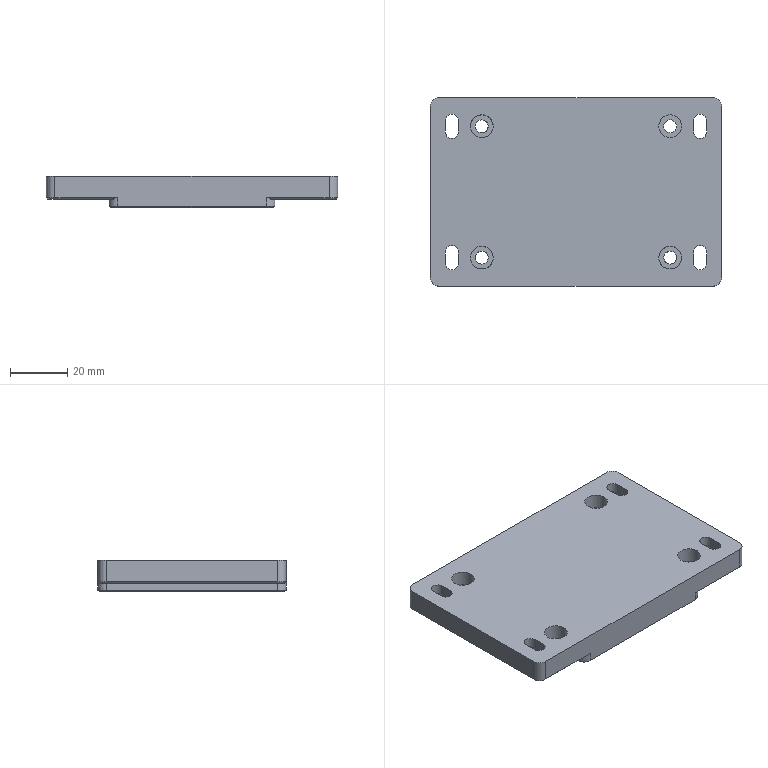CAM job | NX | 3-axis milling, drilling | part box 102 x 66 x 11 mm | stock box 107 x 71 x 15 mm
Tools:
number,name,description,diameter,corner_radius,flute_length,length,flutes
3,D3,平底铣刀-粗,3.0,0.0,20.0,75.0,2
4,D4,平底铣刀-粗,4.0,0.0,25.0,75.0,2
9,D10,平底铣刀-粗,10.0,0.0,35.0,75.0,2
17,D3-J,平底铣刀-精,3.0,0.0,50.0,75.0,2
7,D6-J,平底铣刀-精,6.0,0.0,25.0,75.0,2
10,D10-J,平底铣刀-精,10.0,0.0,35.0,75.0,2
1,D80R0.8飞刀,圆鼻刀-粗,80.0,0.8,50.0,75.0,2
1,D80R0.8飞刀-J,圆鼻刀-精,80.0,0.8,50.0,75.0,2
2,D6倒角刀,倒角刀,6.0,0.0,3.0,25.0,2
11,ZT4.5,钻头,4.5,0.0,35.0,50.0,2
Operations:
program,operation,operation_type,tool,method,geometry_group,spindle_rpm,surface_speed,feed_per_tooth,feed_cut,feed_plunge,cut_length_mm,path_length_mm,cut_time_min,machine_time_min
B,底壁铣飞面一刀开粗_COPY,VolumeBased25DMillingOperation,D80R0.8飞刀,分层开粗-切深K-步距G,W-B,2800.0,703.696,0.5357,3000.0,100.0,1471.358,2844.438,0.4905,0.6278
B,底壁铣飞面一刀精光_COPY,VolumeBased25DMillingOperation,D80R0.8飞刀-J,侧刃精光-切深K-步距G,W-B,4000.0,1005.28,0.125,1000.0,100.0,209.998,245.998,0.21,0.2136
B,底壁铣分层开粗-中_COPY,VolumeBased25DMillingOperation,D10,分层开粗-切深K-步距G,W-B,8000.0,251.32,0.25,4000.0,100.0,3414.944,3835.101,0.8537,0.8958
B,底壁铣螺旋开粗-小_COPY,VolumeBased25DMillingOperation,D4,分层开粗-切深K-步距G,W-B,8000.0,100.528,0.125,2000.0,100.0,1342.105,1728.411,0.6711,0.7097
B,钻倒角_1,Operation,D6倒角刀,METHOD,W-B,8000.0,150.796,0.0625,1000.0,0.0,22.2,257.664,0.0222,0.0457
B,平面去毛刺6X45L_COPY,SurfaceContour,D6倒角刀,爬面_倒角-切深0-步距G,W-B,6500.0,122.519,0.1154,1500.0,100.0,162.118,541.688,0.1081,0.146
B,平面去毛刺6X45L_COPY_1,SurfaceContour,D6倒角刀,爬面_倒角-切深0-步距G,W-B,6500.0,122.519,0.1154,1500.0,100.0,487.503,672.815,0.325,0.3435
B,底壁铣螺旋精光-小_COPY,VolumeBased25DMillingOperation,D3-J,螺旋精光-切深K-步距G,W-B,8000.0,100.528,0.05,800.0,100.0,424.4,802.202,0.5305,0.5683
B,底壁铣精光底面-中_COPY,VolumeBased25DMillingOperation,D6-J,精光步距切深关,W-B,7000.0,175.0,0.0536,1500.0,100.0,985.189,1134.547,0.6568,0.6717
B,等高精光-中_COPY,ZLevelMilling,D6-J,侧刃精光-切深K-步距G,W-B,8000.0,150.792,0.0625,1000.0,100.0,167.935,260.403,0.1679,0.1772
A,顶面,FaceMilling,D80R0.8飞刀,侧刃精光-切深K-步距G,W-A,4000.0,1005.31,0.125,1000.0,100.0,196.0,232.0,0.196,0.1996
A,外形粗_2,VolumeBased25DMillingOperation,D10,METHOD,W-A,8000.0,251.327,0.3125,5000.0,80.0,5807.814,5857.614,1.162,1.167
A,沉头孔打点-深0.8,Operation,D6倒角刀,NONE,W-A,8000.0,150.796,0.0312,500.0,90.0,7.2,215.429,0.0144,0.0352
A,沉头孔-钻孔0段,Operation,ZT4.5,NONE,W-A,2800.0,39.584,0.0179,100.0,90.0,49.408,299.845,0.4941,0.5191
A,通腰槽粗_1,VolumeBased25DMillingOperation,D3,METHOD,W-A,6000.0,75.398,0.1,1200.0,100.0,972.91,1324.611,0.8108,0.8459
A,铣孔开粗D4_1,CylinderMilling,D4,NONE,W-A,8000.0,100.531,0.075,1200.0,100.0,1011.052,1348.652,0.8425,0.8763
A,腰槽精_1,VolumeBased25DMillingOperation,D3-J,METHOD,W-A,6000.0,113.0,0.0417,500.0,100.0,59.763,428.764,0.1195,0.1564
A,铣孔精光D4_1,CylinderMilling,D3-J,精光步距切深关,W-A,8000.0,100.531,0.0312,500.0,100.0,171.867,509.467,0.3437,0.3775
A,仅选体,SurfaceContour,D6倒角刀,METHOD,W-A,8000.0,150.796,0.1875,3000.0,100.0,440.604,844.713,0.1469,0.1873
A,铣倒角_1,PlanarMilling,D6倒角刀,NONE,W-A,8000.0,150.796,0.0312,500.0,100.0,135.871,445.263,0.2717,0.3027
A,外形半精_2,VolumeBased25DMillingOperation,D10-J,METHOD,W-A,8000.0,251.327,0.0625,1000.0,100.0,367.252,428.851,0.3673,0.3734